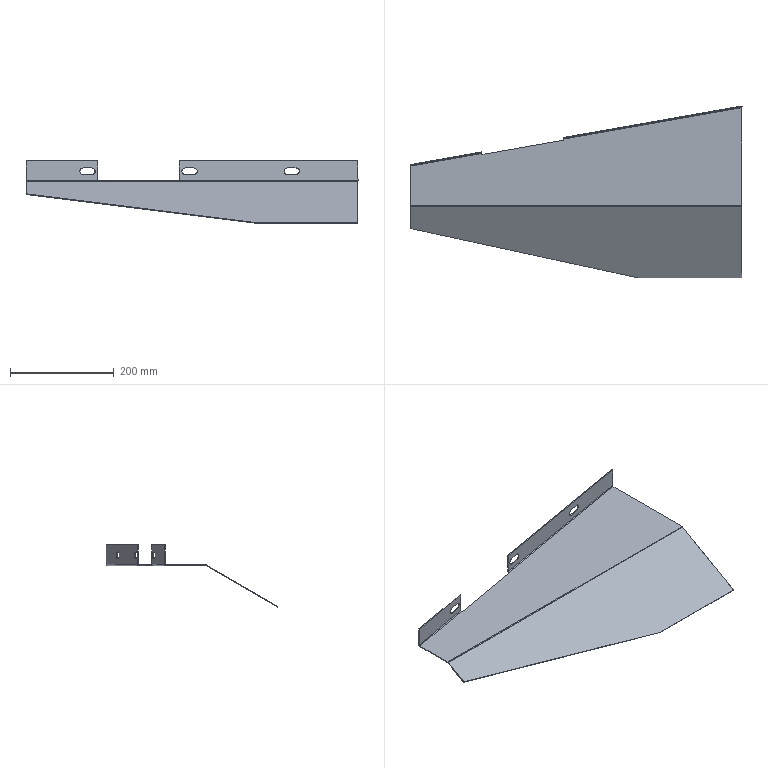Part | SolidWorks | features BaseBody 1 | 1 solid | 42 faces | box 640.37 x 331.413 x 119.799 mm | volume 272644 mm3 | plane 25 | cylinder 15 | spline 2 | commonest cylinder face diameters 13 x9 3 x3 6 x3
STEP:
#1=CARTESIAN_POINT('',(-193.452,62.314,26.5));
#2=VERTEX_POINT('',#1);
#3=CARTESIAN_POINT('',(-187.051,63.443,20.));
#4=VERTEX_POINT('',#3);
#5=CARTESIAN_POINT('',(-193.452,62.314,20.));
#6=DIRECTION('',(-0.1736,0.9848,0.));
#7=DIRECTION('',(0.9848,0.1736,0.));
#8=AXIS2_PLACEMENT_3D('',#5,#6,#7);
#9=CIRCLE('',#8,6.5);
#10=EDGE_CURVE('',#2,#4,#9,.T.);
#11=ORIENTED_EDGE('',*,*,#10,.T.);
#12=CARTESIAN_POINT('',(-186.79,61.965,20.));
#13=VERTEX_POINT('',#12);
#14=CARTESIAN_POINT('',(-187.051,63.443,20.));
#15=DIRECTION('',(0.1736,-0.9848,0.));
#16=VECTOR('',#15,1000.);
#17=LINE('',#14,#16);
#18=EDGE_CURVE('',#4,#13,#17,.T.);
#19=ORIENTED_EDGE('',*,*,#18,.T.);
#20=CARTESIAN_POINT('',(-193.192,60.837,26.5));
#21=VERTEX_POINT('',#20);
#22=CARTESIAN_POINT('',(-193.192,60.837,20.));
#23=DIRECTION('',(-0.1736,0.9848,0.));
#24=DIRECTION('',(0.9848,0.1736,0.));
#25=AXIS2_PLACEMENT_3D('',#22,#23,#24);
#26=CIRCLE('',#25,6.5);
#27=EDGE_CURVE('',#21,#13,#26,.T.);
#28=ORIENTED_EDGE('',*,*,#27,.F.);
#29=CARTESIAN_POINT('',(-193.452,62.314,26.5));
#30=DIRECTION('',(0.1736,-0.9848,0.));
#31=VECTOR('',#30,1000.);
#32=LINE('',#29,#31);
#33=EDGE_CURVE('',#2,#21,#32,.T.);
#34=ORIENTED_EDGE('',*,*,#33,.F.);
#35=EDGE_LOOP('',(#11,#19,#28,#34));
#36=FACE_OUTER_BOUND('',#35,.T.);
#37=CARTESIAN_POINT('',(-193.452,62.314,20.));
#38=DIRECTION('',(0.1736,-0.9848,0.));
#39=DIRECTION('',(0.9848,0.1736,0.));
#40=AXIS2_PLACEMENT_3D('',#37,#38,#39);
#41=CYLINDRICAL_SURFACE('',#40,6.5);
#42=ADVANCED_FACE('',(#36),#41,.F.);
#43=CARTESIAN_POINT('',(3.509,97.043,26.5));
#44=VERTEX_POINT('',#43);
#45=CARTESIAN_POINT('',(9.911,98.172,20.));
#46=VERTEX_POINT('',#45);
#47=CARTESIAN_POINT('',(3.509,97.043,20.));
#48=DIRECTION('',(-0.1736,0.9848,0.));
#49=DIRECTION('',(0.9848,0.1736,0.));
#50=AXIS2_PLACEMENT_3D('',#47,#48,#49);
#51=CIRCLE('',#50,6.5);
#52=EDGE_CURVE('',#44,#46,#51,.T.);
#53=ORIENTED_EDGE('',*,*,#52,.T.);
#54=CARTESIAN_POINT('',(10.171,96.695,20.));
#55=VERTEX_POINT('',#54);
#56=CARTESIAN_POINT('',(9.911,98.172,20.));
#57=DIRECTION('',(0.1736,-0.9848,0.));
#58=VECTOR('',#57,1000.);
#59=LINE('',#56,#58);
#60=EDGE_CURVE('',#46,#55,#59,.T.);
#61=ORIENTED_EDGE('',*,*,#60,.T.);
#62=CARTESIAN_POINT('',(3.77,95.566,26.5));
#63=VERTEX_POINT('',#62);
#64=CARTESIAN_POINT('',(3.77,95.566,20.));
#65=DIRECTION('',(-0.1736,0.9848,0.));
#66=DIRECTION('',(0.9848,0.1736,0.));
#67=AXIS2_PLACEMENT_3D('',#64,#65,#66);
#68=CIRCLE('',#67,6.5);
#69=EDGE_CURVE('',#63,#55,#68,.T.);
#70=ORIENTED_EDGE('',*,*,#69,.F.);
#71=CARTESIAN_POINT('',(3.77,95.566,26.5));
#72=DIRECTION('',(-0.1736,0.9848,0.));
#73=VECTOR('',#72,1000.);
#74=LINE('',#71,#73);
#75=EDGE_CURVE('',#63,#44,#74,.T.);
#76=ORIENTED_EDGE('',*,*,#75,.T.);
#77=EDGE_LOOP('',(#53,#61,#70,#76));
#78=FACE_OUTER_BOUND('',#77,.T.);
#79=CARTESIAN_POINT('',(3.509,97.043,20.));
#80=DIRECTION('',(0.1736,-0.9848,0.));
#81=DIRECTION('',(0.9848,0.1736,0.));
#82=AXIS2_PLACEMENT_3D('',#79,#80,#81);
#83=CYLINDRICAL_SURFACE('',#82,6.5);
#84=ADVANCED_FACE('',(#78),#83,.F.);
#85=CARTESIAN_POINT('',(200.471,131.773,26.5));
#86=VERTEX_POINT('',#85);
#87=CARTESIAN_POINT('',(206.872,132.902,20.));
#88=VERTEX_POINT('',#87);
#89=CARTESIAN_POINT('',(200.471,131.773,20.));
#90=DIRECTION('',(-0.1736,0.9848,0.));
#91=DIRECTION('',(0.9848,0.1736,0.));
#92=AXIS2_PLACEMENT_3D('',#89,#90,#91);
#93=CIRCLE('',#92,6.5);
#94=EDGE_CURVE('',#86,#88,#93,.T.);
#95=ORIENTED_EDGE('',*,*,#94,.T.);
#96=CARTESIAN_POINT('',(207.133,131.425,20.));
#97=VERTEX_POINT('',#96);
#98=CARTESIAN_POINT('',(206.872,132.902,20.));
#99=DIRECTION('',(0.1736,-0.9848,0.));
#100=VECTOR('',#99,1000.);
#101=LINE('',#98,#100);
#102=EDGE_CURVE('',#88,#97,#101,.T.);
#103=ORIENTED_EDGE('',*,*,#102,.T.);
#104=CARTESIAN_POINT('',(200.731,130.296,26.5));
#105=VERTEX_POINT('',#104);
#106=CARTESIAN_POINT('',(200.731,130.296,20.));
#107=DIRECTION('',(-0.1736,0.9848,0.));
#108=DIRECTION('',(0.9848,0.1736,0.));
#109=AXIS2_PLACEMENT_3D('',#106,#107,#108);
#110=CIRCLE('',#109,6.5);
#111=EDGE_CURVE('',#105,#97,#110,.T.);
#112=ORIENTED_EDGE('',*,*,#111,.F.);
#113=CARTESIAN_POINT('',(200.731,130.296,26.5));
#114=DIRECTION('',(-0.1736,0.9848,0.));
#115=VECTOR('',#114,1000.);
#116=LINE('',#113,#115);
#117=EDGE_CURVE('',#105,#86,#116,.T.);
#118=ORIENTED_EDGE('',*,*,#117,.T.);
#119=EDGE_LOOP('',(#95,#103,#112,#118));
#120=FACE_OUTER_BOUND('',#119,.T.);
#121=CARTESIAN_POINT('',(200.471,131.773,20.));
#122=DIRECTION('',(0.1736,-0.9848,0.));
#123=DIRECTION('',(0.9848,0.1736,0.));
#124=AXIS2_PLACEMENT_3D('',#121,#122,#123);
#125=CYLINDRICAL_SURFACE('',#124,6.5);
#126=ADVANCED_FACE('',(#120),#125,.F.);
#127=CARTESIAN_POINT('',(-23.689,87.17,0.));
#128=VERTEX_POINT('',#127);
#129=CARTESIAN_POINT('',(-181.259,59.387,0.));
#130=VERTEX_POINT('',#129);
#131=CARTESIAN_POINT('',(-23.689,87.17,0.));
#132=DIRECTION('',(-0.9848,-0.1736,0.));
#133=VECTOR('',#132,1000.);
#134=LINE('',#131,#133);
#135=EDGE_CURVE('',#128,#130,#134,.T.);
#136=ORIENTED_EDGE('',*,*,#135,.F.);
#137=CARTESIAN_POINT('',(-24.037,89.14,0.));
#138=VERTEX_POINT('',#137);
#139=CARTESIAN_POINT('',(-24.037,89.14,0.));
#140=DIRECTION('',(0.1736,-0.9848,0.));
#141=VECTOR('',#140,1000.);
#142=LINE('',#139,#141);
#143=EDGE_CURVE('',#138,#128,#142,.T.);
#144=ORIENTED_EDGE('',*,*,#143,.F.);
#145=CARTESIAN_POINT('',(320.,149.803,0.));
#146=VERTEX_POINT('',#145);
#147=CARTESIAN_POINT('',(320.,149.803,0.));
#148=DIRECTION('',(-0.9848,-0.1736,0.));
#149=VECTOR('',#148,1000.);
#150=LINE('',#147,#149);
#151=EDGE_CURVE('',#146,#138,#150,.T.);
#152=ORIENTED_EDGE('',*,*,#151,.F.);
#153=CARTESIAN_POINT('',(320.,-39.196,0.));
#154=VERTEX_POINT('',#153);
#155=CARTESIAN_POINT('',(320.,30.681,0.));
#156=DIRECTION('',(0.,1.,0.));
#157=VECTOR('',#156,1000.);
#158=LINE('',#155,#157);
#159=EDGE_CURVE('',#154,#146,#158,.T.);
#160=ORIENTED_EDGE('',*,*,#159,.F.);
#161=CARTESIAN_POINT('',(-320.,-39.196,0.));
#162=VERTEX_POINT('',#161);
#163=CARTESIAN_POINT('',(23.108,-39.196,0.));
#164=DIRECTION('',(1.,0.,0.));
#165=VECTOR('',#164,1000.);
#166=LINE('',#163,#165);
#167=EDGE_CURVE('',#162,#154,#166,.T.);
#168=ORIENTED_EDGE('',*,*,#167,.F.);
#169=CARTESIAN_POINT('',(-320.,36.954,0.));
#170=VERTEX_POINT('',#169);
#171=CARTESIAN_POINT('',(-320.,30.681,0.));
#172=DIRECTION('',(0.,-1.,0.));
#173=VECTOR('',#172,1000.);
#174=LINE('',#171,#173);
#175=EDGE_CURVE('',#170,#162,#174,.T.);
#176=ORIENTED_EDGE('',*,*,#175,.F.);
#177=CARTESIAN_POINT('',(-181.606,61.356,0.));
#178=VERTEX_POINT('',#177);
#179=CARTESIAN_POINT('',(-181.606,61.356,0.));
#180=DIRECTION('',(-0.9848,-0.1736,0.));
#181=VECTOR('',#180,1000.);
#182=LINE('',#179,#181);
#183=EDGE_CURVE('',#178,#170,#182,.T.);
#184=ORIENTED_EDGE('',*,*,#183,.F.);
#185=CARTESIAN_POINT('',(-181.259,59.387,0.));
#186=DIRECTION('',(-0.1736,0.9848,0.));
#187=VECTOR('',#186,1000.);
#188=LINE('',#185,#187);
#189=EDGE_CURVE('',#130,#178,#188,.T.);
#190=ORIENTED_EDGE('',*,*,#189,.F.);
#191=EDGE_LOOP('',(#136,#144,#152,#160,#168,#176,#184,#190));
#192=FACE_OUTER_BOUND('',#191,.T.);
#193=CARTESIAN_POINT('',(23.108,30.681,0.));
#194=DIRECTION('',(0.,0.,1.));
#195=DIRECTION('',(1.,0.,0.));
#196=AXIS2_PLACEMENT_3D('',#193,#194,#195);
#197=PLANE('',#196);
#198=ADVANCED_FACE('',(#192),#197,.F.);
#199=CARTESIAN_POINT('',(-182.127,64.311,3.));
#200=VERTEX_POINT('',#199);
#201=CARTESIAN_POINT('',(-181.606,61.356,3.));
#202=DIRECTION('',(-0.9848,-0.1736,0.));
#203=DIRECTION('',(-0.1736,0.9848,0.));
#204=AXIS2_PLACEMENT_3D('',#201,#202,#203);
#205=CIRCLE('',#204,3.);
#206=EDGE_CURVE('',#200,#178,#205,.T.);
#207=ORIENTED_EDGE('',*,*,#206,.F.);
#208=CARTESIAN_POINT('',(-182.127,64.311,40.));
#209=VERTEX_POINT('',#208);
#210=CARTESIAN_POINT('',(-182.127,64.311,55.));
#211=DIRECTION('',(0.,0.,-1.));
#212=VECTOR('',#211,1000.);
#213=LINE('',#210,#212);
#214=EDGE_CURVE('',#209,#200,#213,.T.);
#215=ORIENTED_EDGE('',*,*,#214,.F.);
#216=CARTESIAN_POINT('',(-181.866,62.834,40.));
#217=VERTEX_POINT('',#216);
#218=CARTESIAN_POINT('',(-181.866,62.834,40.));
#219=DIRECTION('',(-0.1736,0.9848,0.));
#220=VECTOR('',#219,1000.);
#221=LINE('',#218,#220);
#222=EDGE_CURVE('',#217,#209,#221,.T.);
#223=ORIENTED_EDGE('',*,*,#222,.F.);
#224=CARTESIAN_POINT('',(-181.866,62.834,3.));
#225=VERTEX_POINT('',#224);
#226=CARTESIAN_POINT('',(-181.866,62.834,55.));
#227=DIRECTION('',(0.,0.,1.));
#228=VECTOR('',#227,1000.);
#229=LINE('',#226,#228);
#230=EDGE_CURVE('',#225,#217,#229,.T.);
#231=ORIENTED_EDGE('',*,*,#230,.F.);
#232=CARTESIAN_POINT('',(-181.606,61.356,1.5));
#233=VERTEX_POINT('',#232);
#234=CARTESIAN_POINT('',(-181.606,61.356,3.));
#235=DIRECTION('',(0.9848,0.1736,0.));
#236=DIRECTION('',(-0.1736,0.9848,0.));
#237=AXIS2_PLACEMENT_3D('',#234,#235,#236);
#238=CIRCLE('',#237,1.5);
#239=EDGE_CURVE('',#233,#225,#238,.T.);
#240=ORIENTED_EDGE('',*,*,#239,.F.);
#241=CARTESIAN_POINT('',(-181.259,59.387,1.5));
#242=VERTEX_POINT('',#241);
#243=CARTESIAN_POINT('',(-182.127,64.311,1.5));
#244=DIRECTION('',(-0.1736,0.9848,0.));
#245=VECTOR('',#244,1000.);
#246=LINE('',#243,#245);
#247=EDGE_CURVE('',#242,#233,#246,.T.);
#248=ORIENTED_EDGE('',*,*,#247,.F.);
#249=CARTESIAN_POINT('',(-181.259,59.387,55.));
#250=DIRECTION('',(0.,0.,1.));
#251=VECTOR('',#250,1000.);
#252=LINE('',#249,#251);
#253=EDGE_CURVE('',#130,#242,#252,.T.);
#254=ORIENTED_EDGE('',*,*,#253,.F.);
#255=ORIENTED_EDGE('',*,*,#189,.T.);
#256=EDGE_LOOP('',(#207,#215,#223,#231,#240,#248,#254,#255));
#257=FACE_OUTER_BOUND('',#256,.T.);
#258=CARTESIAN_POINT('',(-182.127,64.311,55.));
#259=DIRECTION('',(-0.9848,-0.1736,0.));
#260=DIRECTION('',(0.1736,-0.9848,0.));
#261=AXIS2_PLACEMENT_3D('',#258,#259,#260);
#262=PLANE('',#261);
#263=ADVANCED_FACE('',(#257),#262,.F.);
#264=ORIENTED_EDGE('',*,*,#253,.T.);
#265=CARTESIAN_POINT('',(-23.689,87.17,1.5));
#266=VERTEX_POINT('',#265);
#267=CARTESIAN_POINT('',(-102.474,73.279,1.5));
#268=DIRECTION('',(-0.9848,-0.1736,0.));
#269=VECTOR('',#268,1000.);
#270=LINE('',#267,#269);
#271=EDGE_CURVE('',#266,#242,#270,.T.);
#272=ORIENTED_EDGE('',*,*,#271,.F.);
#273=CARTESIAN_POINT('',(-23.689,87.17,25.));
#274=DIRECTION('',(0.,0.,1.));
#275=VECTOR('',#274,1000.);
#276=LINE('',#273,#275);
#277=EDGE_CURVE('',#128,#266,#276,.T.);
#278=ORIENTED_EDGE('',*,*,#277,.F.);
#279=ORIENTED_EDGE('',*,*,#135,.T.);
#280=EDGE_LOOP('',(#264,#272,#278,#279));
#281=FACE_OUTER_BOUND('',#280,.T.);
#282=CARTESIAN_POINT('',(-102.474,73.279,25.));
#283=DIRECTION('',(0.1736,-0.9848,0.));
#284=DIRECTION('',(0.9848,0.1736,0.));
#285=AXIS2_PLACEMENT_3D('',#282,#283,#284);
#286=PLANE('',#285);
#287=ADVANCED_FACE('',(#281),#286,.F.);
#288=ORIENTED_EDGE('',*,*,#277,.T.);
#289=CARTESIAN_POINT('',(-24.037,89.14,1.5));
#290=VERTEX_POINT('',#289);
#291=CARTESIAN_POINT('',(-24.558,92.094,1.5));
#292=DIRECTION('',(0.1736,-0.9848,0.));
#293=VECTOR('',#292,1000.);
#294=LINE('',#291,#293);
#295=EDGE_CURVE('',#290,#266,#294,.T.);
#296=ORIENTED_EDGE('',*,*,#295,.F.);
#297=CARTESIAN_POINT('',(-24.297,90.617,3.));
#298=VERTEX_POINT('',#297);
#299=CARTESIAN_POINT('',(-24.037,89.14,3.));
#300=DIRECTION('',(-0.9848,-0.1736,0.));
#301=DIRECTION('',(-0.1736,0.9848,0.));
#302=AXIS2_PLACEMENT_3D('',#299,#300,#301);
#303=CIRCLE('',#302,1.5);
#304=EDGE_CURVE('',#298,#290,#303,.T.);
#305=ORIENTED_EDGE('',*,*,#304,.F.);
#306=CARTESIAN_POINT('',(-24.297,90.617,40.));
#307=VERTEX_POINT('',#306);
#308=CARTESIAN_POINT('',(-24.297,90.617,-5.));
#309=DIRECTION('',(0.,0.,-1.));
#310=VECTOR('',#309,1000.);
#311=LINE('',#308,#310);
#312=EDGE_CURVE('',#307,#298,#311,.T.);
#313=ORIENTED_EDGE('',*,*,#312,.F.);
#314=CARTESIAN_POINT('',(-24.558,92.094,40.));
#315=VERTEX_POINT('',#314);
#316=CARTESIAN_POINT('',(-24.558,92.094,40.));
#317=DIRECTION('',(0.1736,-0.9848,0.));
#318=VECTOR('',#317,1000.);
#319=LINE('',#316,#318);
#320=EDGE_CURVE('',#315,#307,#319,.T.);
#321=ORIENTED_EDGE('',*,*,#320,.F.);
#322=CARTESIAN_POINT('',(-24.558,92.094,3.));
#323=VERTEX_POINT('',#322);
#324=CARTESIAN_POINT('',(-24.558,92.094,-5.));
#325=DIRECTION('',(0.,0.,1.));
#326=VECTOR('',#325,1000.);
#327=LINE('',#324,#326);
#328=EDGE_CURVE('',#323,#315,#327,.T.);
#329=ORIENTED_EDGE('',*,*,#328,.F.);
#330=CARTESIAN_POINT('',(-24.037,89.14,3.));
#331=DIRECTION('',(0.9848,0.1736,0.));
#332=DIRECTION('',(-0.1736,0.9848,0.));
#333=AXIS2_PLACEMENT_3D('',#330,#331,#332);
#334=CIRCLE('',#333,3.);
#335=EDGE_CURVE('',#138,#323,#334,.T.);
#336=ORIENTED_EDGE('',*,*,#335,.F.);
#337=ORIENTED_EDGE('',*,*,#143,.T.);
#338=EDGE_LOOP('',(#288,#296,#305,#313,#321,#329,#336,#337));
#339=FACE_OUTER_BOUND('',#338,.T.);
#340=CARTESIAN_POINT('',(-24.558,92.094,-5.));
#341=DIRECTION('',(0.9848,0.1736,0.));
#342=DIRECTION('',(-0.1736,0.9848,0.));
#343=AXIS2_PLACEMENT_3D('',#340,#341,#342);
#344=PLANE('',#343);
#345=ADVANCED_FACE('',(#339),#344,.F.);
#346=CARTESIAN_POINT('',(320.,152.849,3.));
#347=VERTEX_POINT('',#346);
#348=CARTESIAN_POINT('',(320.,152.849,3.));
#349=CARTESIAN_POINT('',(319.978,152.845,2.802));
#350=CARTESIAN_POINT('',(319.96,152.822,2.607));
#351=CARTESIAN_POINT('',(319.93,152.739,2.221));
#352=CARTESIAN_POINT('',(319.918,152.678,2.031));
#353=CARTESIAN_POINT('',(319.901,152.523,1.67));
#354=CARTESIAN_POINT('',(319.895,152.429,1.497));
#355=CARTESIAN_POINT('',(319.89,152.205,1.169));
#356=CARTESIAN_POINT('',(319.89,152.078,1.017));
#357=CARTESIAN_POINT('',(319.894,151.798,0.7407));
#358=CARTESIAN_POINT('',(319.899,151.644,0.6153));
#359=CARTESIAN_POINT('',(319.912,151.314,0.3961));
#360=CARTESIAN_POINT('',(319.921,151.14,0.3041));
#361=CARTESIAN_POINT('',(319.94,150.777,0.1542));
#362=CARTESIAN_POINT('',(319.952,150.585,0.09621));
#363=CARTESIAN_POINT('',(319.975,150.198,0.01942));
#364=CARTESIAN_POINT('',(319.988,150.002,0.));
#365=CARTESIAN_POINT('',(320.,149.803,0.));
#366=B_SPLINE_CURVE_WITH_KNOTS('',3,(#348,#349,#350,#351,#352,#353,#354,#355,#356,#357,#358,#359,#360,#361,#362,#363,#364,#365),.UNSPECIFIED.,.F.,.F.,(4,2,2,2,2,2,2,2,4),(0.,0.000592,0.001184,0.001776,0.002368,0.00296,0.003552,0.004144,0.004736),.UNSPECIFIED.);
#367=EDGE_CURVE('',#347,#146,#366,.T.);
#368=ORIENTED_EDGE('',*,*,#367,.T.);
#369=ORIENTED_EDGE('',*,*,#151,.T.);
#370=ORIENTED_EDGE('',*,*,#335,.T.);
#371=CARTESIAN_POINT('',(-0.5209,96.333,3.));
#372=DIRECTION('',(0.9848,0.1736,0.));
#373=VECTOR('',#372,1000.);
#374=LINE('',#371,#373);
#375=EDGE_CURVE('',#323,#347,#374,.T.);
#376=ORIENTED_EDGE('',*,*,#375,.T.);
#377=EDGE_LOOP('',(#368,#369,#370,#376));
#378=FACE_OUTER_BOUND('',#377,.T.);
#379=CARTESIAN_POINT('',(0.,93.378,3.));
#380=DIRECTION('',(0.9848,0.1736,0.));
#381=DIRECTION('',(-0.1736,0.9848,0.));
#382=AXIS2_PLACEMENT_3D('',#379,#380,#381);
#383=CYLINDRICAL_SURFACE('',#382,3.);
#384=ADVANCED_FACE('',(#378),#383,.T.);
#385=CARTESIAN_POINT('',(320.,149.803,1.5));
#386=VERTEX_POINT('',#385);
#387=CARTESIAN_POINT('',(320.,149.803,0.));
#388=DIRECTION('',(0.,0.,1.));
#389=VECTOR('',#388,1000.);
#390=LINE('',#387,#389);
#391=EDGE_CURVE('',#146,#386,#390,.T.);
#392=ORIENTED_EDGE('',*,*,#391,.T.);
#393=CARTESIAN_POINT('',(320.,-39.196,1.5));
#394=VERTEX_POINT('',#393);
#395=CARTESIAN_POINT('',(320.,40.,1.5));
#396=DIRECTION('',(0.,-1.,0.));
#397=VECTOR('',#396,1000.);
#398=LINE('',#395,#397);
#399=EDGE_CURVE('',#386,#394,#398,.T.);
#400=ORIENTED_EDGE('',*,*,#399,.T.);
#401=CARTESIAN_POINT('',(320.,-40.696,1.098));
#402=VERTEX_POINT('',#401);
#403=CARTESIAN_POINT('',(320.,-39.196,-1.5));
#404=DIRECTION('',(1.,0.,0.));
#405=DIRECTION('',(0.,1.,0.));
#406=AXIS2_PLACEMENT_3D('',#403,#404,#405);
#407=CIRCLE('',#406,3.);
#408=EDGE_CURVE('',#394,#402,#407,.T.);
#409=ORIENTED_EDGE('',*,*,#408,.T.);
#410=CARTESIAN_POINT('',(320.,-178.564,-78.5));
#411=VERTEX_POINT('',#410);
#412=CARTESIAN_POINT('',(320.,-40.696,1.098));
#413=DIRECTION('',(0.,-0.866,-0.5));
#414=VECTOR('',#413,1000.);
#415=LINE('',#412,#414);
#416=EDGE_CURVE('',#402,#411,#415,.T.);
#417=ORIENTED_EDGE('',*,*,#416,.T.);
#418=CARTESIAN_POINT('',(320.,-177.814,-79.799));
#419=VERTEX_POINT('',#418);
#420=CARTESIAN_POINT('',(320.,-178.564,-78.5));
#421=DIRECTION('',(0.,0.5,-0.866));
#422=VECTOR('',#421,1000.);
#423=LINE('',#420,#422);
#424=EDGE_CURVE('',#411,#419,#423,.T.);
#425=ORIENTED_EDGE('',*,*,#424,.T.);
#426=CARTESIAN_POINT('',(320.,-39.946,-0.201));
#427=VERTEX_POINT('',#426);
#428=CARTESIAN_POINT('',(320.,-108.39,-39.717));
#429=DIRECTION('',(0.,0.866,0.5));
#430=VECTOR('',#429,1000.);
#431=LINE('',#428,#430);
#432=EDGE_CURVE('',#419,#427,#431,.T.);
#433=ORIENTED_EDGE('',*,*,#432,.T.);
#434=CARTESIAN_POINT('',(320.,-39.196,-1.5));
#435=DIRECTION('',(-1.,0.,0.));
#436=DIRECTION('',(0.,1.,0.));
#437=AXIS2_PLACEMENT_3D('',#434,#435,#436);
#438=CIRCLE('',#437,1.5);
#439=EDGE_CURVE('',#427,#154,#438,.T.);
#440=ORIENTED_EDGE('',*,*,#439,.T.);
#441=ORIENTED_EDGE('',*,*,#159,.T.);
#442=EDGE_LOOP('',(#392,#400,#409,#417,#425,#433,#440,#441));
#443=FACE_OUTER_BOUND('',#442,.T.);
#444=CARTESIAN_POINT('',(320.,40.,0.));
#445=DIRECTION('',(1.,0.,0.));
#446=DIRECTION('',(0.,0.,-1.));
#447=AXIS2_PLACEMENT_3D('',#444,#445,#446);
#448=PLANE('',#447);
#449=ADVANCED_FACE('',(#443),#448,.T.);
#450=CARTESIAN_POINT('',(-320.,-39.946,-0.201));
#451=VERTEX_POINT('',#450);
#452=CARTESIAN_POINT('',(-320.,-39.196,-1.5));
#453=DIRECTION('',(1.,0.,0.));
#454=DIRECTION('',(0.,1.,0.));
#455=AXIS2_PLACEMENT_3D('',#452,#453,#454);
#456=CIRCLE('',#455,1.5);
#457=EDGE_CURVE('',#162,#451,#456,.T.);
#458=ORIENTED_EDGE('',*,*,#457,.F.);
#459=ORIENTED_EDGE('',*,*,#167,.T.);
#460=ORIENTED_EDGE('',*,*,#439,.F.);
#461=CARTESIAN_POINT('',(0.,-39.946,-0.201));
#462=DIRECTION('',(1.,0.,0.));
#463=VECTOR('',#462,1000.);
#464=LINE('',#461,#463);
#465=EDGE_CURVE('',#451,#427,#464,.T.);
#466=ORIENTED_EDGE('',*,*,#465,.F.);
#467=EDGE_LOOP('',(#458,#459,#460,#466));
#468=FACE_OUTER_BOUND('',#467,.T.);
#469=CARTESIAN_POINT('',(0.,-39.196,-1.5));
#470=DIRECTION('',(1.,0.,0.));
#471=DIRECTION('',(0.,1.,0.));
#472=AXIS2_PLACEMENT_3D('',#469,#470,#471);
#473=CYLINDRICAL_SURFACE('',#472,1.5);
#474=ADVANCED_FACE('',(#468),#473,.F.);
#475=CARTESIAN_POINT('',(-320.,36.954,1.5));
#476=VERTEX_POINT('',#475);
#477=CARTESIAN_POINT('',(-320.,36.954,0.75));
#478=DIRECTION('',(0.,0.,1.));
#479=VECTOR('',#478,1000.);
#480=LINE('',#477,#479);
#481=EDGE_CURVE('',#170,#476,#480,.T.);
#482=ORIENTED_EDGE('',*,*,#481,.F.);
#483=ORIENTED_EDGE('',*,*,#175,.T.);
#484=ORIENTED_EDGE('',*,*,#457,.T.);
#485=CARTESIAN_POINT('',(-320.,-82.551,-24.799));
#486=VERTEX_POINT('',#485);
#487=CARTESIAN_POINT('',(-320.,-108.39,-39.717));
#488=DIRECTION('',(0.,-0.866,-0.5));
#489=VECTOR('',#488,1000.);
#490=LINE('',#487,#489);
#491=EDGE_CURVE('',#451,#486,#490,.T.);
#492=ORIENTED_EDGE('',*,*,#491,.T.);
#493=CARTESIAN_POINT('',(-320.,-83.301,-23.5));
#494=VERTEX_POINT('',#493);
#495=CARTESIAN_POINT('',(-320.,-83.301,-23.5));
#496=DIRECTION('',(0.,-0.5,0.866));
#497=VECTOR('',#496,1000.);
#498=LINE('',#495,#497);
#499=EDGE_CURVE('',#486,#494,#498,.T.);
#500=ORIENTED_EDGE('',*,*,#499,.T.);
#501=CARTESIAN_POINT('',(-320.,-40.696,1.098));
#502=VERTEX_POINT('',#501);
#503=CARTESIAN_POINT('',(-320.,-83.301,-23.5));
#504=DIRECTION('',(0.,0.866,0.5));
#505=VECTOR('',#504,1000.);
#506=LINE('',#503,#505);
#507=EDGE_CURVE('',#494,#502,#506,.T.);
#508=ORIENTED_EDGE('',*,*,#507,.T.);
#509=CARTESIAN_POINT('',(-320.,-39.196,1.5));
#510=VERTEX_POINT('',#509);
#511=CARTESIAN_POINT('',(-320.,-39.196,-1.5));
#512=DIRECTION('',(-1.,0.,0.));
#513=DIRECTION('',(0.,1.,0.));
#514=AXIS2_PLACEMENT_3D('',#511,#512,#513);
#515=CIRCLE('',#514,3.);
#516=EDGE_CURVE('',#502,#510,#515,.T.);
#517=ORIENTED_EDGE('',*,*,#516,.T.);
#518=CARTESIAN_POINT('',(-320.,-40.,1.5));
#519=DIRECTION('',(0.,1.,0.));
#520=VECTOR('',#519,1000.);
#521=LINE('',#518,#520);
#522=EDGE_CURVE('',#510,#476,#521,.T.);
#523=ORIENTED_EDGE('',*,*,#522,.T.);
#524=EDGE_LOOP('',(#482,#483,#484,#492,#500,#508,#517,#523));
#525=FACE_OUTER_BOUND('',#524,.T.);
#526=CARTESIAN_POINT('',(-320.,-40.,0.));
#527=DIRECTION('',(-1.,0.,0.));
#528=DIRECTION('',(0.,-1.,0.));
#529=AXIS2_PLACEMENT_3D('',#526,#527,#528);
#530=PLANE('',#529);
#531=ADVANCED_FACE('',(#525),#530,.T.);
#532=CARTESIAN_POINT('',(-320.,40.,3.));
#533=VERTEX_POINT('',#532);
#534=CARTESIAN_POINT('',(-320.,36.954,0.));
#535=CARTESIAN_POINT('',(-320.012,37.153,0.));
#536=CARTESIAN_POINT('',(-320.025,37.349,0.01942));
#537=CARTESIAN_POINT('',(-320.048,37.736,0.09615));
#538=CARTESIAN_POINT('',(-320.06,37.927,0.1542));
#539=CARTESIAN_POINT('',(-320.079,38.291,0.3041));
#540=CARTESIAN_POINT('',(-320.088,38.464,0.3961));
#541=CARTESIAN_POINT('',(-320.101,38.795,0.6151));
#542=CARTESIAN_POINT('',(-320.106,38.949,0.7406));
#543=CARTESIAN_POINT('',(-320.11,39.228,1.017));
#544=CARTESIAN_POINT('',(-320.11,39.356,1.169));
#545=CARTESIAN_POINT('',(-320.105,39.579,1.497));
#546=CARTESIAN_POINT('',(-320.099,39.674,1.67));
#547=CARTESIAN_POINT('',(-320.082,39.829,2.031));
#548=CARTESIAN_POINT('',(-320.07,39.89,2.221));
#549=CARTESIAN_POINT('',(-320.04,39.973,2.607));
#550=CARTESIAN_POINT('',(-320.022,39.996,2.802));
#551=CARTESIAN_POINT('',(-320.,40.,3.));
#552=B_SPLINE_CURVE_WITH_KNOTS('',3,(#534,#535,#536,#537,#538,#539,#540,#541,#542,#543,#544,#545,#546,#547,#548,#549,#550,#551),.UNSPECIFIED.,.F.,.F.,(4,2,2,2,2,2,2,2,4),(0.,0.000592,0.001184,0.001776,0.002368,0.00296,0.003552,0.004144,0.004736),.UNSPECIFIED.);
#553=EDGE_CURVE('',#170,#533,#552,.T.);
#554=ORIENTED_EDGE('',*,*,#553,.T.);
#555=CARTESIAN_POINT('',(-0.5209,96.333,3.));
#556=DIRECTION('',(0.9848,0.1736,0.));
#557=VECTOR('',#556,1000.);
#558=LINE('',#555,#557);
#559=EDGE_CURVE('',#533,#200,#558,.T.);
#560=ORIENTED_EDGE('',*,*,#559,.T.);
#561=ORIENTED_EDGE('',*,*,#206,.T.);
#562=ORIENTED_EDGE('',*,*,#183,.T.);
#563=EDGE_LOOP('',(#554,#560,#561,#562));
#564=FACE_OUTER_BOUND('',#563,.T.);
#565=CARTESIAN_POINT('',(0.,93.378,3.));
#566=DIRECTION('',(0.9848,0.1736,0.));
#567=DIRECTION('',(-0.1736,0.9848,0.));
#568=AXIS2_PLACEMENT_3D('',#565,#566,#567);
#569=CYLINDRICAL_SURFACE('',#568,3.);
#570=ADVANCED_FACE('',(#564),#569,.T.);
#571=CARTESIAN_POINT('',(-210.194,59.362,26.5));
#572=VERTEX_POINT('',#571);
#573=CARTESIAN_POINT('',(-0.2465,96.381,26.5));
#574=DIRECTION('',(0.9848,0.1736,0.));
#575=VECTOR('',#574,1000.);
#576=LINE('',#573,#575);
#577=EDGE_CURVE('',#572,#2,#576,.T.);
#578=ORIENTED_EDGE('',*,*,#577,.F.);
#579=CARTESIAN_POINT('',(-210.194,59.362,13.5));
#580=VERTEX_POINT('',#579);
#581=CARTESIAN_POINT('',(-210.194,59.362,20.));
#582=DIRECTION('',(-0.1736,0.9848,0.));
#583=DIRECTION('',(0.9848,0.1736,0.));
#584=AXIS2_PLACEMENT_3D('',#581,#582,#583);
#585=CIRCLE('',#584,6.5);
#586=EDGE_CURVE('',#580,#572,#585,.T.);
#587=ORIENTED_EDGE('',*,*,#586,.F.);
#588=CARTESIAN_POINT('',(-193.452,62.314,13.5));
#589=VERTEX_POINT('',#588);
#590=CARTESIAN_POINT('',(-0.2465,96.381,13.5));
#591=DIRECTION('',(-0.9848,-0.1736,0.));
#592=VECTOR('',#591,1000.);
#593=LINE('',#590,#592);
#594=EDGE_CURVE('',#589,#580,#593,.T.);
#595=ORIENTED_EDGE('',*,*,#594,.F.);
#596=CARTESIAN_POINT('',(-193.452,62.314,20.));
#597=DIRECTION('',(-0.1736,0.9848,0.));
#598=DIRECTION('',(0.9848,0.1736,0.));
#599=AXIS2_PLACEMENT_3D('',#596,#597,#598);
#600=CIRCLE('',#599,6.5);
#601=EDGE_CURVE('',#4,#589,#600,.T.);
#602=ORIENTED_EDGE('',*,*,#601,.F.);
#603=ORIENTED_EDGE('',*,*,#10,.F.);
#604=EDGE_LOOP('',(#578,#587,#595,#602,#603));
#605=FACE_BOUND('',#604,.T.);
#606=ORIENTED_EDGE('',*,*,#559,.F.);
#607=CARTESIAN_POINT('',(-320.,40.,40.));
#608=VERTEX_POINT('',#607);
#609=CARTESIAN_POINT('',(-320.,40.,19.802));
#610=DIRECTION('',(0.,0.,-1.));
#611=VECTOR('',#610,1000.);
#612=LINE('',#609,#611);
#613=EDGE_CURVE('',#608,#533,#612,.T.);
#614=ORIENTED_EDGE('',*,*,#613,.F.);
#615=CARTESIAN_POINT('',(-0.2465,96.381,40.));
#616=DIRECTION('',(-0.9848,-0.1736,0.));
#617=VECTOR('',#616,1000.);
#618=LINE('',#615,#617);
#619=EDGE_CURVE('',#209,#608,#618,.T.);
#620=ORIENTED_EDGE('',*,*,#619,.F.);
#621=ORIENTED_EDGE('',*,*,#214,.T.);
#622=EDGE_LOOP('',(#606,#614,#620,#621));
#623=FACE_OUTER_BOUND('',#622,.T.);
#624=CARTESIAN_POINT('',(-0.2465,96.381,19.802));
#625=DIRECTION('',(0.1736,-0.9848,0.));
#626=DIRECTION('',(0.9848,0.1736,0.));
#627=AXIS2_PLACEMENT_3D('',#624,#625,#626);
#628=PLANE('',#627);
#629=ADVANCED_FACE('',(#605,#623),#628,.F.);
#630=CARTESIAN_POINT('',(-209.933,57.885,13.5));
#631=VERTEX_POINT('',#630);
#632=CARTESIAN_POINT('',(-209.933,57.885,26.5));
#633=VERTEX_POINT('',#632);
#634=CARTESIAN_POINT('',(-209.933,57.885,20.));
#635=DIRECTION('',(-0.1736,0.9848,0.));
#636=DIRECTION('',(0.9848,0.1736,0.));
#637=AXIS2_PLACEMENT_3D('',#634,#635,#636);
#638=CIRCLE('',#637,6.5);
#639=EDGE_CURVE('',#631,#633,#638,.T.);
#640=ORIENTED_EDGE('',*,*,#639,.T.);
#641=CARTESIAN_POINT('',(0.01396,94.904,26.5));
#642=DIRECTION('',(0.9848,0.1736,0.));
#643=VECTOR('',#642,1000.);
#644=LINE('',#641,#643);
#645=EDGE_CURVE('',#633,#21,#644,.T.);
#646=ORIENTED_EDGE('',*,*,#645,.T.);
#647=ORIENTED_EDGE('',*,*,#27,.T.);
#648=CARTESIAN_POINT('',(-193.192,60.837,13.5));
#649=VERTEX_POINT('',#648);
#650=CARTESIAN_POINT('',(-193.192,60.837,20.));
#651=DIRECTION('',(-0.1736,0.9848,0.));
#652=DIRECTION('',(0.9848,0.1736,0.));
#653=AXIS2_PLACEMENT_3D('',#650,#651,#652);
#654=CIRCLE('',#653,6.5);
#655=EDGE_CURVE('',#13,#649,#654,.T.);
#656=ORIENTED_EDGE('',*,*,#655,.T.);
#657=CARTESIAN_POINT('',(0.01396,94.904,13.5));
#658=DIRECTION('',(-0.9848,-0.1736,0.));
#659=VECTOR('',#658,1000.);
#660=LINE('',#657,#659);
#661=EDGE_CURVE('',#649,#631,#660,.T.);
#662=ORIENTED_EDGE('',*,*,#661,.T.);
#663=EDGE_LOOP('',(#640,#646,#647,#656,#662));
#664=FACE_BOUND('',#663,.T.);
#665=CARTESIAN_POINT('',(-319.74,38.523,40.));
#666=VERTEX_POINT('',#665);
#667=CARTESIAN_POINT('',(-319.74,38.523,3.));
#668=VERTEX_POINT('',#667);
#669=CARTESIAN_POINT('',(-319.74,38.523,19.802));
#670=DIRECTION('',(0.,0.,-1.));
#671=VECTOR('',#670,1000.);
#672=LINE('',#669,#671);
#673=EDGE_CURVE('',#666,#668,#672,.T.);
#674=ORIENTED_EDGE('',*,*,#673,.T.);
#675=CARTESIAN_POINT('',(0.01396,94.904,3.));
#676=DIRECTION('',(0.9848,0.1736,0.));
#677=VECTOR('',#676,1000.);
#678=LINE('',#675,#677);
#679=EDGE_CURVE('',#668,#225,#678,.T.);
#680=ORIENTED_EDGE('',*,*,#679,.T.);
#681=ORIENTED_EDGE('',*,*,#230,.T.);
#682=CARTESIAN_POINT('',(0.01396,94.904,40.));
#683=DIRECTION('',(-0.9848,-0.1736,0.));
#684=VECTOR('',#683,1000.);
#685=LINE('',#682,#684);
#686=EDGE_CURVE('',#217,#666,#685,.T.);
#687=ORIENTED_EDGE('',*,*,#686,.T.);
#688=EDGE_LOOP('',(#674,#680,#681,#687));
#689=FACE_OUTER_BOUND('',#688,.T.);
#690=CARTESIAN_POINT('',(0.01396,94.904,19.802));
#691=DIRECTION('',(0.1736,-0.9848,0.));
#692=DIRECTION('',(0.9848,0.1736,0.));
#693=AXIS2_PLACEMENT_3D('',#690,#691,#692);
#694=PLANE('',#693);
#695=ADVANCED_FACE('',(#664,#689),#694,.T.);
#696=ORIENTED_EDGE('',*,*,#679,.F.);
#697=CARTESIAN_POINT('',(-320.,36.954,1.5));
#698=CARTESIAN_POINT('',(-319.991,37.157,1.5));
#699=CARTESIAN_POINT('',(-319.981,37.355,1.539));
#700=CARTESIAN_POINT('',(-319.964,37.635,1.652));
#701=CARTESIAN_POINT('',(-319.957,37.724,1.698));
#702=CARTESIAN_POINT('',(-319.942,37.892,1.806));
#703=CARTESIAN_POINT('',(-319.933,37.972,1.87));
#704=CARTESIAN_POINT('',(-319.914,38.116,2.008));
#705=CARTESIAN_POINT('',(-319.903,38.181,2.084));
#706=CARTESIAN_POINT('',(-319.879,38.296,2.247));
#707=CARTESIAN_POINT('',(-319.865,38.346,2.335));
#708=CARTESIAN_POINT('',(-319.82,38.468,2.605));
#709=CARTESIAN_POINT('',(-319.783,38.515,2.802));
#710=CARTESIAN_POINT('',(-319.74,38.523,3.));
#711=B_SPLINE_CURVE_WITH_KNOTS('',3,(#697,#698,#699,#700,#701,#702,#703,#704,#705,#706,#707,#708,#709,#710),.UNSPECIFIED.,.F.,.F.,(4,2,2,2,2,2,4),(0.,0.0006004,0.0009005,0.001201,0.001501,0.001801,0.002401),.UNSPECIFIED.);
#712=EDGE_CURVE('',#476,#668,#711,.T.);
#713=ORIENTED_EDGE('',*,*,#712,.F.);
#714=CARTESIAN_POINT('',(0.,93.378,1.5));
#715=DIRECTION('',(-0.9848,-0.1736,0.));
#716=VECTOR('',#715,1000.);
#717=LINE('',#714,#716);
#718=EDGE_CURVE('',#233,#476,#717,.T.);
#719=ORIENTED_EDGE('',*,*,#718,.F.);
#720=ORIENTED_EDGE('',*,*,#239,.T.);
#721=EDGE_LOOP('',(#696,#713,#719,#720));
#722=FACE_OUTER_BOUND('',#721,.T.);
#723=CARTESIAN_POINT('',(0.,93.378,3.));
#724=DIRECTION('',(0.9848,0.1736,0.));
#725=DIRECTION('',(-0.1736,0.9848,0.));
#726=AXIS2_PLACEMENT_3D('',#723,#724,#725);
#727=CYLINDRICAL_SURFACE('',#726,1.5);
#728=ADVANCED_FACE('',(#722),#727,.F.);
#729=ORIENTED_EDGE('',*,*,#295,.T.);
#730=ORIENTED_EDGE('',*,*,#271,.T.);
#731=ORIENTED_EDGE('',*,*,#247,.T.);
#732=ORIENTED_EDGE('',*,*,#718,.T.);
#733=ORIENTED_EDGE('',*,*,#522,.F.);
#734=CARTESIAN_POINT('',(23.108,-39.196,1.5));
#735=DIRECTION('',(1.,0.,0.));
#736=VECTOR('',#735,1000.);
#737=LINE('',#734,#736);
#738=EDGE_CURVE('',#510,#394,#737,.T.);
#739=ORIENTED_EDGE('',*,*,#738,.T.);
#740=ORIENTED_EDGE('',*,*,#399,.F.);
#741=CARTESIAN_POINT('',(320.,149.803,1.5));
#742=DIRECTION('',(-0.9848,-0.1736,0.));
#743=VECTOR('',#742,1000.);
#744=LINE('',#741,#743);
#745=EDGE_CURVE('',#386,#290,#744,.T.);
#746=ORIENTED_EDGE('',*,*,#745,.T.);
#747=EDGE_LOOP('',(#729,#730,#731,#732,#733,#739,#740,#746));
#748=FACE_OUTER_BOUND('',#747,.T.);
#749=CARTESIAN_POINT('',(23.108,30.681,1.5));
#750=DIRECTION('',(0.,0.,1.));
#751=DIRECTION('',(1.,0.,0.));
#752=AXIS2_PLACEMENT_3D('',#749,#750,#751);
#753=PLANE('',#752);
#754=ADVANCED_FACE('',(#748),#753,.T.);
#755=ORIENTED_EDGE('',*,*,#745,.F.);
#756=CARTESIAN_POINT('',(320.26,151.372,3.));
#757=VERTEX_POINT('',#756);
#758=CARTESIAN_POINT('',(320.26,151.372,3.));
#759=CARTESIAN_POINT('',(320.217,151.364,2.802));
#760=CARTESIAN_POINT('',(320.18,151.318,2.608));
#761=CARTESIAN_POINT('',(320.135,151.196,2.335));
#762=CARTESIAN_POINT('',(320.121,151.147,2.249));
#763=CARTESIAN_POINT('',(320.097,151.032,2.086));
#764=CARTESIAN_POINT('',(320.086,150.966,2.009));
#765=CARTESIAN_POINT('',(320.067,150.822,1.87));
#766=CARTESIAN_POINT('',(320.058,150.744,1.808));
#767=CARTESIAN_POINT('',(320.043,150.575,1.699));
#768=CARTESIAN_POINT('',(320.036,150.485,1.652));
#769=CARTESIAN_POINT('',(320.019,150.207,1.54));
#770=CARTESIAN_POINT('',(320.009,150.006,1.5));
#771=CARTESIAN_POINT('',(320.,149.803,1.5));
#772=B_SPLINE_CURVE_WITH_KNOTS('',3,(#758,#759,#760,#761,#762,#763,#764,#765,#766,#767,#768,#769,#770,#771),.UNSPECIFIED.,.F.,.F.,(4,2,2,2,2,2,4),(0.,0.0006004,0.0009006,0.001201,0.001501,0.001801,0.002401),.UNSPECIFIED.);
#773=EDGE_CURVE('',#757,#386,#772,.T.);
#774=ORIENTED_EDGE('',*,*,#773,.F.);
#775=CARTESIAN_POINT('',(-0.2605,94.856,3.));
#776=DIRECTION('',(0.9848,0.1736,0.));
#777=VECTOR('',#776,1000.);
#778=LINE('',#775,#777);
#779=EDGE_CURVE('',#298,#757,#778,.T.);
#780=ORIENTED_EDGE('',*,*,#779,.F.);
#781=ORIENTED_EDGE('',*,*,#304,.T.);
#782=EDGE_LOOP('',(#755,#774,#780,#781));
#783=FACE_OUTER_BOUND('',#782,.T.);
#784=CARTESIAN_POINT('',(0.,93.378,3.));
#785=DIRECTION('',(0.9848,0.1736,0.));
#786=DIRECTION('',(-0.1736,0.9848,0.));
#787=AXIS2_PLACEMENT_3D('',#784,#785,#786);
#788=CYLINDRICAL_SURFACE('',#787,1.5);
#789=ADVANCED_FACE('',(#783),#788,.F.);
#790=CARTESIAN_POINT('',(-12.972,92.614,13.5));
#791=VERTEX_POINT('',#790);
#792=CARTESIAN_POINT('',(-12.972,92.614,26.5));
#793=VERTEX_POINT('',#792);
#794=CARTESIAN_POINT('',(-12.972,92.614,20.));
#795=DIRECTION('',(-0.1736,0.9848,0.));
#796=DIRECTION('',(0.9848,0.1736,0.));
#797=AXIS2_PLACEMENT_3D('',#794,#795,#796);
#798=CIRCLE('',#797,6.5);
#799=EDGE_CURVE('',#791,#793,#798,.T.);
#800=ORIENTED_EDGE('',*,*,#799,.T.);
#801=CARTESIAN_POINT('',(0.01396,94.904,26.5));
#802=DIRECTION('',(0.9848,0.1736,0.));
#803=VECTOR('',#802,1000.);
#804=LINE('',#801,#803);
#805=EDGE_CURVE('',#793,#63,#804,.T.);
#806=ORIENTED_EDGE('',*,*,#805,.T.);
#807=ORIENTED_EDGE('',*,*,#69,.T.);
#808=CARTESIAN_POINT('',(3.77,95.566,13.5));
#809=VERTEX_POINT('',#808);
#810=CARTESIAN_POINT('',(3.77,95.566,20.));
#811=DIRECTION('',(-0.1736,0.9848,0.));
#812=DIRECTION('',(0.9848,0.1736,0.));
#813=AXIS2_PLACEMENT_3D('',#810,#811,#812);
#814=CIRCLE('',#813,6.5);
#815=EDGE_CURVE('',#55,#809,#814,.T.);
#816=ORIENTED_EDGE('',*,*,#815,.T.);
#817=CARTESIAN_POINT('',(0.01396,94.904,13.5));
#818=DIRECTION('',(-0.9848,-0.1736,0.));
#819=VECTOR('',#818,1000.);
#820=LINE('',#817,#819);
#821=EDGE_CURVE('',#809,#791,#820,.T.);
#822=ORIENTED_EDGE('',*,*,#821,.T.);
#823=EDGE_LOOP('',(#800,#806,#807,#816,#822));
#824=FACE_BOUND('',#823,.T.);
#825=CARTESIAN_POINT('',(183.99,127.344,13.5));
#826=VERTEX_POINT('',#825);
#827=CARTESIAN_POINT('',(183.99,127.344,26.5));
#828=VERTEX_POINT('',#827);
#829=CARTESIAN_POINT('',(183.99,127.344,20.));
#830=DIRECTION('',(-0.1736,0.9848,0.));
#831=DIRECTION('',(0.9848,0.1736,0.));
#832=AXIS2_PLACEMENT_3D('',#829,#830,#831);
#833=CIRCLE('',#832,6.5);
#834=EDGE_CURVE('',#826,#828,#833,.T.);
#835=ORIENTED_EDGE('',*,*,#834,.T.);
#836=CARTESIAN_POINT('',(0.01396,94.904,26.5));
#837=DIRECTION('',(0.9848,0.1736,0.));
#838=VECTOR('',#837,1000.);
#839=LINE('',#836,#838);
#840=EDGE_CURVE('',#828,#105,#839,.T.);
#841=ORIENTED_EDGE('',*,*,#840,.T.);
#842=ORIENTED_EDGE('',*,*,#111,.T.);
#843=CARTESIAN_POINT('',(200.731,130.296,13.5));
#844=VERTEX_POINT('',#843);
#845=CARTESIAN_POINT('',(200.731,130.296,20.));
#846=DIRECTION('',(-0.1736,0.9848,0.));
#847=DIRECTION('',(0.9848,0.1736,0.));
#848=AXIS2_PLACEMENT_3D('',#845,#846,#847);
#849=CIRCLE('',#848,6.5);
#850=EDGE_CURVE('',#97,#844,#849,.T.);
#851=ORIENTED_EDGE('',*,*,#850,.T.);
#852=CARTESIAN_POINT('',(0.01396,94.904,13.5));
#853=DIRECTION('',(-0.9848,-0.1736,0.));
#854=VECTOR('',#853,1000.);
#855=LINE('',#852,#854);
#856=EDGE_CURVE('',#844,#826,#855,.T.);
#857=ORIENTED_EDGE('',*,*,#856,.T.);
#858=EDGE_LOOP('',(#835,#841,#842,#851,#857));
#859=FACE_BOUND('',#858,.T.);
#860=CARTESIAN_POINT('',(320.26,151.372,40.));
#861=VERTEX_POINT('',#860);
#862=CARTESIAN_POINT('',(320.26,151.372,19.802));
#863=DIRECTION('',(0.,0.,1.));
#864=VECTOR('',#863,1000.);
#865=LINE('',#862,#864);
#866=EDGE_CURVE('',#757,#861,#865,.T.);
#867=ORIENTED_EDGE('',*,*,#866,.T.);
#868=CARTESIAN_POINT('',(0.01396,94.904,40.));
#869=DIRECTION('',(-0.9848,-0.1736,0.));
#870=VECTOR('',#869,1000.);
#871=LINE('',#868,#870);
#872=EDGE_CURVE('',#861,#307,#871,.T.);
#873=ORIENTED_EDGE('',*,*,#872,.T.);
#874=ORIENTED_EDGE('',*,*,#312,.T.);
#875=ORIENTED_EDGE('',*,*,#779,.T.);
#876=EDGE_LOOP('',(#867,#873,#874,#875));
#877=FACE_OUTER_BOUND('',#876,.T.);
#878=CARTESIAN_POINT('',(0.01396,94.904,19.802));
#879=DIRECTION('',(0.1736,-0.9848,0.));
#880=DIRECTION('',(0.9848,0.1736,0.));
#881=AXIS2_PLACEMENT_3D('',#878,#879,#880);
#882=PLANE('',#881);
#883=ADVANCED_FACE('',(#824,#859,#877),#882,.T.);
#884=CARTESIAN_POINT('',(-13.232,94.091,26.5));
#885=VERTEX_POINT('',#884);
#886=CARTESIAN_POINT('',(-0.2465,96.381,26.5));
#887=DIRECTION('',(0.9848,0.1736,0.));
#888=VECTOR('',#887,1000.);
#889=LINE('',#886,#888);
#890=EDGE_CURVE('',#885,#44,#889,.T.);
#891=ORIENTED_EDGE('',*,*,#890,.F.);
#892=CARTESIAN_POINT('',(-13.232,94.091,13.5));
#893=VERTEX_POINT('',#892);
#894=CARTESIAN_POINT('',(-13.232,94.091,20.));
#895=DIRECTION('',(-0.1736,0.9848,0.));
#896=DIRECTION('',(0.9848,0.1736,0.));
#897=AXIS2_PLACEMENT_3D('',#894,#895,#896);
#898=CIRCLE('',#897,6.5);
#899=EDGE_CURVE('',#893,#885,#898,.T.);
#900=ORIENTED_EDGE('',*,*,#899,.F.);
#901=CARTESIAN_POINT('',(3.509,97.043,13.5));
#902=VERTEX_POINT('',#901);
#903=CARTESIAN_POINT('',(-0.2465,96.381,13.5));
#904=DIRECTION('',(-0.9848,-0.1736,0.));
#905=VECTOR('',#904,1000.);
#906=LINE('',#903,#905);
#907=EDGE_CURVE('',#902,#893,#906,.T.);
#908=ORIENTED_EDGE('',*,*,#907,.F.);
#909=CARTESIAN_POINT('',(3.509,97.043,20.));
#910=DIRECTION('',(-0.1736,0.9848,0.));
#911=DIRECTION('',(0.9848,0.1736,0.));
#912=AXIS2_PLACEMENT_3D('',#909,#910,#911);
#913=CIRCLE('',#912,6.5);
#914=EDGE_CURVE('',#46,#902,#913,.T.);
#915=ORIENTED_EDGE('',*,*,#914,.F.);
#916=ORIENTED_EDGE('',*,*,#52,.F.);
#917=EDGE_LOOP('',(#891,#900,#908,#915,#916));
#918=FACE_BOUND('',#917,.T.);
#919=CARTESIAN_POINT('',(183.729,128.821,26.5));
#920=VERTEX_POINT('',#919);
#921=CARTESIAN_POINT('',(-0.2465,96.381,26.5));
#922=DIRECTION('',(0.9848,0.1736,0.));
#923=VECTOR('',#922,1000.);
#924=LINE('',#921,#923);
#925=EDGE_CURVE('',#920,#86,#924,.T.);
#926=ORIENTED_EDGE('',*,*,#925,.F.);
#927=CARTESIAN_POINT('',(183.729,128.821,13.5));
#928=VERTEX_POINT('',#927);
#929=CARTESIAN_POINT('',(183.729,128.821,20.));
#930=DIRECTION('',(-0.1736,0.9848,0.));
#931=DIRECTION('',(0.9848,0.1736,0.));
#932=AXIS2_PLACEMENT_3D('',#929,#930,#931);
#933=CIRCLE('',#932,6.5);
#934=EDGE_CURVE('',#928,#920,#933,.T.);
#935=ORIENTED_EDGE('',*,*,#934,.F.);
#936=CARTESIAN_POINT('',(200.471,131.773,13.5));
#937=VERTEX_POINT('',#936);
#938=CARTESIAN_POINT('',(-0.2465,96.381,13.5));
#939=DIRECTION('',(-0.9848,-0.1736,0.));
#940=VECTOR('',#939,1000.);
#941=LINE('',#938,#940);
#942=EDGE_CURVE('',#937,#928,#941,.T.);
#943=ORIENTED_EDGE('',*,*,#942,.F.);
#944=CARTESIAN_POINT('',(200.471,131.773,20.));
#945=DIRECTION('',(-0.1736,0.9848,0.));
#946=DIRECTION('',(0.9848,0.1736,0.));
#947=AXIS2_PLACEMENT_3D('',#944,#945,#946);
#948=CIRCLE('',#947,6.5);
#949=EDGE_CURVE('',#88,#937,#948,.T.);
#950=ORIENTED_EDGE('',*,*,#949,.F.);
#951=ORIENTED_EDGE('',*,*,#94,.F.);
#952=EDGE_LOOP('',(#926,#935,#943,#950,#951));
#953=FACE_BOUND('',#952,.T.);
#954=CARTESIAN_POINT('',(320.,152.849,40.));
#955=VERTEX_POINT('',#954);
#956=CARTESIAN_POINT('',(-0.2465,96.381,40.));
#957=DIRECTION('',(-0.9848,-0.1736,0.));
#958=VECTOR('',#957,1000.);
#959=LINE('',#956,#958);
#960=EDGE_CURVE('',#955,#315,#959,.T.);
#961=ORIENTED_EDGE('',*,*,#960,.F.);
#962=CARTESIAN_POINT('',(320.,152.849,19.802));
#963=DIRECTION('',(0.,0.,1.));
#964=VECTOR('',#963,1000.);
#965=LINE('',#962,#964);
#966=EDGE_CURVE('',#347,#955,#965,.T.);
#967=ORIENTED_EDGE('',*,*,#966,.F.);
#968=ORIENTED_EDGE('',*,*,#375,.F.);
#969=ORIENTED_EDGE('',*,*,#328,.T.);
#970=EDGE_LOOP('',(#961,#967,#968,#969));
#971=FACE_OUTER_BOUND('',#970,.T.);
#972=CARTESIAN_POINT('',(-0.2465,96.381,19.802));
#973=DIRECTION('',(0.1736,-0.9848,0.));
#974=DIRECTION('',(0.9848,0.1736,0.));
#975=AXIS2_PLACEMENT_3D('',#972,#973,#974);
#976=PLANE('',#975);
#977=ADVANCED_FACE('',(#918,#953,#971),#976,.F.);
#978=ORIENTED_EDGE('',*,*,#391,.F.);
#979=ORIENTED_EDGE('',*,*,#367,.F.);
#980=CARTESIAN_POINT('',(320.13,152.111,3.));
#981=DIRECTION('',(0.1736,-0.9848,0.));
#982=VECTOR('',#981,1000.);
#983=LINE('',#980,#982);
#984=EDGE_CURVE('',#347,#757,#983,.T.);
#985=ORIENTED_EDGE('',*,*,#984,.T.);
#986=ORIENTED_EDGE('',*,*,#773,.T.);
#987=EDGE_LOOP('',(#978,#979,#985,#986));
#988=FACE_OUTER_BOUND('',#987,.T.);
#989=CARTESIAN_POINT('',(320.,149.803,1.515));
#990=CARTESIAN_POINT('',(320.017,150.144,1.515));
#991=CARTESIAN_POINT('',(320.055,150.941,1.787));
#992=CARTESIAN_POINT('',(320.164,151.34,2.556));
#993=CARTESIAN_POINT('',(320.263,151.357,3.));
#994=CARTESIAN_POINT('',(320.,149.803,1.51));
#995=CARTESIAN_POINT('',(320.016,150.145,1.51));
#996=CARTESIAN_POINT('',(320.054,150.945,1.783));
#997=CARTESIAN_POINT('',(320.163,151.345,2.554));
#998=CARTESIAN_POINT('',(320.262,151.362,3.));
#999=CARTESIAN_POINT('',(320.,149.803,1.505));
#1000=CARTESIAN_POINT('',(320.016,150.146,1.505));
#1001=CARTESIAN_POINT('',(320.054,150.949,1.779));
#1002=CARTESIAN_POINT('',(320.162,151.35,2.553));
#1003=CARTESIAN_POINT('',(320.261,151.367,3.));
#1004=CARTESIAN_POINT('',(320.,149.803,1.5));
#1005=CARTESIAN_POINT('',(320.016,150.148,1.5));
#1006=CARTESIAN_POINT('',(320.053,150.953,1.775));
#1007=CARTESIAN_POINT('',(320.161,151.355,2.551));
#1008=CARTESIAN_POINT('',(320.26,151.372,3.));
#1009=CARTESIAN_POINT('',(320.,149.803,1.));
#1010=CARTESIAN_POINT('',(319.996,150.258,1.));
#1011=CARTESIAN_POINT('',(319.988,151.321,1.366));
#1012=CARTESIAN_POINT('',(320.074,151.847,2.402));
#1013=CARTESIAN_POINT('',(320.174,151.864,3.));
#1014=CARTESIAN_POINT('',(320.,149.803,0.5));
#1015=CARTESIAN_POINT('',(319.977,150.369,0.5));
#1016=CARTESIAN_POINT('',(319.923,151.69,0.9577));
#1017=CARTESIAN_POINT('',(319.988,152.339,2.252));
#1018=CARTESIAN_POINT('',(320.087,152.357,3.));
#1019=CARTESIAN_POINT('',(320.,149.803,0.));
#1020=CARTESIAN_POINT('',(319.958,150.479,0.));
#1021=CARTESIAN_POINT('',(319.858,152.059,0.5492));
#1022=CARTESIAN_POINT('',(319.901,152.832,2.102));
#1023=CARTESIAN_POINT('',(320.,152.849,3.));
#1024=CARTESIAN_POINT('',(320.,149.803,-0.00525));
#1025=CARTESIAN_POINT('',(319.957,150.48,-0.00525));
#1026=CARTESIAN_POINT('',(319.857,152.062,0.5449));
#1027=CARTESIAN_POINT('',(319.9,152.837,2.101));
#1028=CARTESIAN_POINT('',(319.999,152.854,3.));
#1029=CARTESIAN_POINT('',(320.,149.803,-0.0105));
#1030=CARTESIAN_POINT('',(319.957,150.481,-0.0105));
#1031=CARTESIAN_POINT('',(319.857,152.066,0.5406));
#1032=CARTESIAN_POINT('',(319.899,152.842,2.099));
#1033=CARTESIAN_POINT('',(319.998,152.86,3.));
#1034=CARTESIAN_POINT('',(320.,149.803,-0.01575));
#1035=CARTESIAN_POINT('',(319.957,150.483,-0.01575));
#1036=CARTESIAN_POINT('',(319.856,152.07,0.5363));
#1037=CARTESIAN_POINT('',(319.898,152.847,2.098));
#1038=CARTESIAN_POINT('',(319.997,152.865,3.));
#1039=B_SPLINE_SURFACE_WITH_KNOTS('',3,3,((#989,#990,#991,#992,#993),(#994,#995,#996,#997,#998),(#999,#1000,#1001,#1002,#1003),(#1004,#1005,#1006,#1007,#1008),(#1009,#1010,#1011,#1012,#1013),(#1014,#1015,#1016,#1017,#1018),(#1019,#1020,#1021,#1022,#1023),(#1024,#1025,#1026,#1027,#1028),(#1029,#1030,#1031,#1032,#1033),(#1034,#1035,#1036,#1037,#1038)),.UNSPECIFIED.,.F.,.F.,.F.,(4,3,3,4),(4,1,4),(-0.001516,0.,0.15,0.1516),(0.,0.1472,0.3434),.UNSPECIFIED.);
#1040=ADVANCED_FACE('',(#988),#1039,.T.);
#1041=ORIENTED_EDGE('',*,*,#491,.F.);
#1042=ORIENTED_EDGE('',*,*,#465,.T.);
#1043=ORIENTED_EDGE('',*,*,#432,.F.);
#1044=CARTESIAN_POINT('',(120.,-177.814,-79.799));
#1045=VERTEX_POINT('',#1044);
#1046=CARTESIAN_POINT('',(0.,-177.814,-79.799));
#1047=DIRECTION('',(1.,0.,0.));
#1048=VECTOR('',#1047,1000.);
#1049=LINE('',#1046,#1048);
#1050=EDGE_CURVE('',#1045,#419,#1049,.T.);
#1051=ORIENTED_EDGE('',*,*,#1050,.F.);
#1052=CARTESIAN_POINT('',(-320.,-82.551,-24.799));
#1053=DIRECTION('',(0.9701,-0.21,-0.1213));
#1054=VECTOR('',#1053,1000.);
#1055=LINE('',#1052,#1054);
#1056=EDGE_CURVE('',#486,#1045,#1055,.T.);
#1057=ORIENTED_EDGE('',*,*,#1056,.F.);
#1058=EDGE_LOOP('',(#1041,#1042,#1043,#1051,#1057));
#1059=FACE_OUTER_BOUND('',#1058,.T.);
#1060=CARTESIAN_POINT('',(0.,-108.39,-39.717));
#1061=DIRECTION('',(0.,-0.5,0.866));
#1062=DIRECTION('',(0.,-0.866,-0.5));
#1063=AXIS2_PLACEMENT_3D('',#1060,#1061,#1062);
#1064=PLANE('',#1063);
#1065=ADVANCED_FACE('',(#1059),#1064,.F.);
#1066=ORIENTED_EDGE('',*,*,#712,.T.);
#1067=CARTESIAN_POINT('',(-319.87,39.261,3.));
#1068=DIRECTION('',(-0.1736,0.9848,0.));
#1069=VECTOR('',#1068,1000.);
#1070=LINE('',#1067,#1069);
#1071=EDGE_CURVE('',#668,#533,#1070,.T.);
#1072=ORIENTED_EDGE('',*,*,#1071,.T.);
#1073=ORIENTED_EDGE('',*,*,#553,.F.);
#1074=ORIENTED_EDGE('',*,*,#481,.T.);
#1075=EDGE_LOOP('',(#1066,#1072,#1073,#1074));
#1076=FACE_OUTER_BOUND('',#1075,.T.);
#1077=CARTESIAN_POINT('',(-320.,36.954,-0.01578));
#1078=CARTESIAN_POINT('',(-320.043,37.633,-0.01578));
#1079=CARTESIAN_POINT('',(-320.144,39.221,0.5363));
#1080=CARTESIAN_POINT('',(-320.102,39.998,2.098));
#1081=CARTESIAN_POINT('',(-320.003,40.016,3.));
#1082=CARTESIAN_POINT('',(-320.,36.954,-0.01052));
#1083=CARTESIAN_POINT('',(-320.043,37.632,-0.01052));
#1084=CARTESIAN_POINT('',(-320.143,39.217,0.5406));
#1085=CARTESIAN_POINT('',(-320.101,39.993,2.099));
#1086=CARTESIAN_POINT('',(-320.002,40.01,3.));
#1087=CARTESIAN_POINT('',(-320.,36.954,-0.005261));
#1088=CARTESIAN_POINT('',(-320.043,37.631,-0.005261));
#1089=CARTESIAN_POINT('',(-320.143,39.213,0.5449));
#1090=CARTESIAN_POINT('',(-320.1,39.988,2.101));
#1091=CARTESIAN_POINT('',(-320.001,40.005,3.));
#1092=CARTESIAN_POINT('',(-320.,36.954,0.));
#1093=CARTESIAN_POINT('',(-320.042,37.63,0.));
#1094=CARTESIAN_POINT('',(-320.142,39.209,0.5492));
#1095=CARTESIAN_POINT('',(-320.099,39.983,2.102));
#1096=CARTESIAN_POINT('',(-320.,40.,3.));
#1097=CARTESIAN_POINT('',(-320.,36.954,0.5));
#1098=CARTESIAN_POINT('',(-320.023,37.519,0.5));
#1099=CARTESIAN_POINT('',(-320.077,38.841,0.9577));
#1100=CARTESIAN_POINT('',(-320.012,39.49,2.252));
#1101=CARTESIAN_POINT('',(-319.913,39.508,3.));
#1102=CARTESIAN_POINT('',(-320.,36.954,1.));
#1103=CARTESIAN_POINT('',(-320.004,37.409,1.));
#1104=CARTESIAN_POINT('',(-320.012,38.472,1.366));
#1105=CARTESIAN_POINT('',(-319.926,38.998,2.402));
#1106=CARTESIAN_POINT('',(-319.826,39.015,3.));
#1107=CARTESIAN_POINT('',(-320.,36.954,1.5));
#1108=CARTESIAN_POINT('',(-319.984,37.298,1.5));
#1109=CARTESIAN_POINT('',(-319.947,38.103,1.775));
#1110=CARTESIAN_POINT('',(-319.839,38.505,2.551));
#1111=CARTESIAN_POINT('',(-319.74,38.523,3.));
#1112=CARTESIAN_POINT('',(-320.,36.954,1.505));
#1113=CARTESIAN_POINT('',(-319.984,37.297,1.505));
#1114=CARTESIAN_POINT('',(-319.946,38.1,1.779));
#1115=CARTESIAN_POINT('',(-319.838,38.5,2.553));
#1116=CARTESIAN_POINT('',(-319.739,38.518,3.));
#1117=CARTESIAN_POINT('',(-320.,36.954,1.51));
#1118=CARTESIAN_POINT('',(-319.984,37.296,1.51));
#1119=CARTESIAN_POINT('',(-319.946,38.096,1.783));
#1120=CARTESIAN_POINT('',(-319.837,38.495,2.554));
#1121=CARTESIAN_POINT('',(-319.738,38.513,3.));
#1122=CARTESIAN_POINT('',(-320.,36.954,1.515));
#1123=CARTESIAN_POINT('',(-319.983,37.295,1.515));
#1124=CARTESIAN_POINT('',(-319.945,38.092,1.787));
#1125=CARTESIAN_POINT('',(-319.836,38.49,2.556));
#1126=CARTESIAN_POINT('',(-319.737,38.508,3.));
#1127=B_SPLINE_SURFACE_WITH_KNOTS('',3,3,((#1077,#1078,#1079,#1080,#1081),(#1082,#1083,#1084,#1085,#1086),(#1087,#1088,#1089,#1090,#1091),(#1092,#1093,#1094,#1095,#1096),(#1097,#1098,#1099,#1100,#1101),(#1102,#1103,#1104,#1105,#1106),(#1107,#1108,#1109,#1110,#1111),(#1112,#1113,#1114,#1115,#1116),(#1117,#1118,#1119,#1120,#1121),(#1122,#1123,#1124,#1125,#1126)),.UNSPECIFIED.,.F.,.F.,.F.,(4,3,3,4),(4,1,4),(-0.1516,-0.15,0.,0.001516),(-0.3434,-0.1962,0.),.UNSPECIFIED.);
#1128=ADVANCED_FACE('',(#1076),#1127,.T.);
#1129=ORIENTED_EDGE('',*,*,#18,.F.);
#1130=ORIENTED_EDGE('',*,*,#601,.T.);
#1131=CARTESIAN_POINT('',(-193.452,62.314,13.5));
#1132=DIRECTION('',(-0.1736,0.9848,0.));
#1133=VECTOR('',#1132,1000.);
#1134=LINE('',#1131,#1133);
#1135=EDGE_CURVE('',#649,#589,#1134,.T.);
#1136=ORIENTED_EDGE('',*,*,#1135,.F.);
#1137=ORIENTED_EDGE('',*,*,#655,.F.);
#1138=EDGE_LOOP('',(#1129,#1130,#1136,#1137));
#1139=FACE_OUTER_BOUND('',#1138,.T.);
#1140=CARTESIAN_POINT('',(-193.452,62.314,20.));
#1141=DIRECTION('',(0.1736,-0.9848,0.));
#1142=DIRECTION('',(0.9848,0.1736,0.));
#1143=AXIS2_PLACEMENT_3D('',#1140,#1141,#1142);
#1144=CYLINDRICAL_SURFACE('',#1143,6.5);
#1145=ADVANCED_FACE('',(#1139),#1144,.F.);
#1146=CARTESIAN_POINT('',(-210.194,59.362,26.5));
#1147=DIRECTION('',(0.1736,-0.9848,0.));
#1148=VECTOR('',#1147,1000.);
#1149=LINE('',#1146,#1148);
#1150=EDGE_CURVE('',#572,#633,#1149,.T.);
#1151=ORIENTED_EDGE('',*,*,#1150,.F.);
#1152=ORIENTED_EDGE('',*,*,#577,.T.);
#1153=ORIENTED_EDGE('',*,*,#33,.T.);
#1154=ORIENTED_EDGE('',*,*,#645,.F.);
#1155=EDGE_LOOP('',(#1151,#1152,#1153,#1154));
#1156=FACE_OUTER_BOUND('',#1155,.T.);
#1157=CARTESIAN_POINT('',(-193.452,62.314,26.5));
#1158=DIRECTION('',(0.,0.,1.));
#1159=DIRECTION('',(1.,0.,0.));
#1160=AXIS2_PLACEMENT_3D('',#1157,#1158,#1159);
#1161=PLANE('',#1160);
#1162=ADVANCED_FACE('',(#1156),#1161,.F.);
#1163=CARTESIAN_POINT('',(-210.194,59.362,13.5));
#1164=DIRECTION('',(0.1736,-0.9848,0.));
#1165=VECTOR('',#1164,1000.);
#1166=LINE('',#1163,#1165);
#1167=EDGE_CURVE('',#580,#631,#1166,.T.);
#1168=ORIENTED_EDGE('',*,*,#1167,.F.);
#1169=ORIENTED_EDGE('',*,*,#586,.T.);
#1170=ORIENTED_EDGE('',*,*,#1150,.T.);
#1171=ORIENTED_EDGE('',*,*,#639,.F.);
#1172=EDGE_LOOP('',(#1168,#1169,#1170,#1171));
#1173=FACE_OUTER_BOUND('',#1172,.T.);
#1174=CARTESIAN_POINT('',(-210.194,59.362,20.));
#1175=DIRECTION('',(0.1736,-0.9848,0.));
#1176=DIRECTION('',(0.9848,0.1736,0.));
#1177=AXIS2_PLACEMENT_3D('',#1174,#1175,#1176);
#1178=CYLINDRICAL_SURFACE('',#1177,6.5);
#1179=ADVANCED_FACE('',(#1173),#1178,.F.);
#1180=ORIENTED_EDGE('',*,*,#1135,.T.);
#1181=ORIENTED_EDGE('',*,*,#594,.T.);
#1182=ORIENTED_EDGE('',*,*,#1167,.T.);
#1183=ORIENTED_EDGE('',*,*,#661,.F.);
#1184=EDGE_LOOP('',(#1180,#1181,#1182,#1183));
#1185=FACE_OUTER_BOUND('',#1184,.T.);
#1186=CARTESIAN_POINT('',(-210.194,59.362,13.5));
#1187=DIRECTION('',(0.,0.,-1.));
#1188=DIRECTION('',(-1.,0.,0.));
#1189=AXIS2_PLACEMENT_3D('',#1186,#1187,#1188);
#1190=PLANE('',#1189);
#1191=ADVANCED_FACE('',(#1185),#1190,.F.);
#1192=ORIENTED_EDGE('',*,*,#673,.F.);
#1193=CARTESIAN_POINT('',(-319.74,38.523,40.));
#1194=DIRECTION('',(-0.1736,0.9848,0.));
#1195=VECTOR('',#1194,1000.);
#1196=LINE('',#1193,#1195);
#1197=EDGE_CURVE('',#666,#608,#1196,.T.);
#1198=ORIENTED_EDGE('',*,*,#1197,.T.);
#1199=ORIENTED_EDGE('',*,*,#613,.T.);
#1200=ORIENTED_EDGE('',*,*,#1071,.F.);
#1201=EDGE_LOOP('',(#1192,#1198,#1199,#1200));
#1202=FACE_OUTER_BOUND('',#1201,.T.);
#1203=CARTESIAN_POINT('',(-319.74,38.523,40.));
#1204=DIRECTION('',(-0.9848,-0.1736,0.));
#1205=DIRECTION('',(0.1736,-0.9848,0.));
#1206=AXIS2_PLACEMENT_3D('',#1203,#1204,#1205);
#1207=PLANE('',#1206);
#1208=ADVANCED_FACE('',(#1202),#1207,.T.);
#1209=ORIENTED_EDGE('',*,*,#1197,.F.);
#1210=ORIENTED_EDGE('',*,*,#686,.F.);
#1211=ORIENTED_EDGE('',*,*,#222,.T.);
#1212=ORIENTED_EDGE('',*,*,#619,.T.);
#1213=EDGE_LOOP('',(#1209,#1210,#1211,#1212));
#1214=FACE_OUTER_BOUND('',#1213,.T.);
#1215=CARTESIAN_POINT('',(320.26,151.372,40.));
#1216=DIRECTION('',(0.,0.,1.));
#1217=DIRECTION('',(0.,-1.,0.));
#1218=AXIS2_PLACEMENT_3D('',#1215,#1216,#1217);
#1219=PLANE('',#1218);
#1220=ADVANCED_FACE('',(#1214),#1219,.T.);
#1221=ORIENTED_EDGE('',*,*,#738,.F.);
#1222=ORIENTED_EDGE('',*,*,#516,.F.);
#1223=CARTESIAN_POINT('',(0.,-40.696,1.098));
#1224=DIRECTION('',(1.,0.,0.));
#1225=VECTOR('',#1224,1000.);
#1226=LINE('',#1223,#1225);
#1227=EDGE_CURVE('',#502,#402,#1226,.T.);
#1228=ORIENTED_EDGE('',*,*,#1227,.T.);
#1229=ORIENTED_EDGE('',*,*,#408,.F.);
#1230=EDGE_LOOP('',(#1221,#1222,#1228,#1229));
#1231=FACE_OUTER_BOUND('',#1230,.T.);
#1232=CARTESIAN_POINT('',(0.,-39.196,-1.5));
#1233=DIRECTION('',(1.,0.,0.));
#1234=DIRECTION('',(0.,1.,0.));
#1235=AXIS2_PLACEMENT_3D('',#1232,#1233,#1234);
#1236=CYLINDRICAL_SURFACE('',#1235,3.);
#1237=ADVANCED_FACE('',(#1231),#1236,.T.);
#1238=CARTESIAN_POINT('',(-13.232,94.091,26.5));
#1239=DIRECTION('',(0.1736,-0.9848,0.));
#1240=VECTOR('',#1239,1000.);
#1241=LINE('',#1238,#1240);
#1242=EDGE_CURVE('',#885,#793,#1241,.T.);
#1243=ORIENTED_EDGE('',*,*,#1242,.F.);
#1244=ORIENTED_EDGE('',*,*,#890,.T.);
#1245=ORIENTED_EDGE('',*,*,#75,.F.);
#1246=ORIENTED_EDGE('',*,*,#805,.F.);
#1247=EDGE_LOOP('',(#1243,#1244,#1245,#1246));
#1248=FACE_OUTER_BOUND('',#1247,.T.);
#1249=CARTESIAN_POINT('',(3.509,97.043,26.5));
#1250=DIRECTION('',(0.,0.,1.));
#1251=DIRECTION('',(1.,0.,0.));
#1252=AXIS2_PLACEMENT_3D('',#1249,#1250,#1251);
#1253=PLANE('',#1252);
#1254=ADVANCED_FACE('',(#1248),#1253,.F.);
#1255=CARTESIAN_POINT('',(-13.232,94.091,13.5));
#1256=DIRECTION('',(0.1736,-0.9848,0.));
#1257=VECTOR('',#1256,1000.);
#1258=LINE('',#1255,#1257);
#1259=EDGE_CURVE('',#893,#791,#1258,.T.);
#1260=ORIENTED_EDGE('',*,*,#1259,.F.);
#1261=ORIENTED_EDGE('',*,*,#899,.T.);
#1262=ORIENTED_EDGE('',*,*,#1242,.T.);
#1263=ORIENTED_EDGE('',*,*,#799,.F.);
#1264=EDGE_LOOP('',(#1260,#1261,#1262,#1263));
#1265=FACE_OUTER_BOUND('',#1264,.T.);
#1266=CARTESIAN_POINT('',(-13.232,94.091,20.));
#1267=DIRECTION('',(0.1736,-0.9848,0.));
#1268=DIRECTION('',(0.9848,0.1736,0.));
#1269=AXIS2_PLACEMENT_3D('',#1266,#1267,#1268);
#1270=CYLINDRICAL_SURFACE('',#1269,6.5);
#1271=ADVANCED_FACE('',(#1265),#1270,.F.);
#1272=CARTESIAN_POINT('',(3.509,97.043,13.5));
#1273=DIRECTION('',(0.1736,-0.9848,0.));
#1274=VECTOR('',#1273,1000.);
#1275=LINE('',#1272,#1274);
#1276=EDGE_CURVE('',#902,#809,#1275,.T.);
#1277=ORIENTED_EDGE('',*,*,#1276,.F.);
#1278=ORIENTED_EDGE('',*,*,#907,.T.);
#1279=ORIENTED_EDGE('',*,*,#1259,.T.);
#1280=ORIENTED_EDGE('',*,*,#821,.F.);
#1281=EDGE_LOOP('',(#1277,#1278,#1279,#1280));
#1282=FACE_OUTER_BOUND('',#1281,.T.);
#1283=CARTESIAN_POINT('',(-13.232,94.091,13.5));
#1284=DIRECTION('',(0.,0.,-1.));
#1285=DIRECTION('',(-1.,0.,0.));
#1286=AXIS2_PLACEMENT_3D('',#1283,#1284,#1285);
#1287=PLANE('',#1286);
#1288=ADVANCED_FACE('',(#1282),#1287,.F.);
#1289=ORIENTED_EDGE('',*,*,#60,.F.);
#1290=ORIENTED_EDGE('',*,*,#914,.T.);
#1291=ORIENTED_EDGE('',*,*,#1276,.T.);
#1292=ORIENTED_EDGE('',*,*,#815,.F.);
#1293=EDGE_LOOP('',(#1289,#1290,#1291,#1292));
#1294=FACE_OUTER_BOUND('',#1293,.T.);
#1295=CARTESIAN_POINT('',(3.509,97.043,20.));
#1296=DIRECTION('',(0.1736,-0.9848,0.));
#1297=DIRECTION('',(0.9848,0.1736,0.));
#1298=AXIS2_PLACEMENT_3D('',#1295,#1296,#1297);
#1299=CYLINDRICAL_SURFACE('',#1298,6.5);
#1300=ADVANCED_FACE('',(#1294),#1299,.F.);
#1301=CARTESIAN_POINT('',(183.729,128.821,26.5));
#1302=DIRECTION('',(0.1736,-0.9848,0.));
#1303=VECTOR('',#1302,1000.);
#1304=LINE('',#1301,#1303);
#1305=EDGE_CURVE('',#920,#828,#1304,.T.);
#1306=ORIENTED_EDGE('',*,*,#1305,.F.);
#1307=ORIENTED_EDGE('',*,*,#925,.T.);
#1308=ORIENTED_EDGE('',*,*,#117,.F.);
#1309=ORIENTED_EDGE('',*,*,#840,.F.);
#1310=EDGE_LOOP('',(#1306,#1307,#1308,#1309));
#1311=FACE_OUTER_BOUND('',#1310,.T.);
#1312=CARTESIAN_POINT('',(200.471,131.773,26.5));
#1313=DIRECTION('',(0.,0.,1.));
#1314=DIRECTION('',(1.,0.,0.));
#1315=AXIS2_PLACEMENT_3D('',#1312,#1313,#1314);
#1316=PLANE('',#1315);
#1317=ADVANCED_FACE('',(#1311),#1316,.F.);
#1318=CARTESIAN_POINT('',(183.729,128.821,13.5));
#1319=DIRECTION('',(0.1736,-0.9848,0.));
#1320=VECTOR('',#1319,1000.);
#1321=LINE('',#1318,#1320);
#1322=EDGE_CURVE('',#928,#826,#1321,.T.);
#1323=ORIENTED_EDGE('',*,*,#1322,.F.);
#1324=ORIENTED_EDGE('',*,*,#934,.T.);
#1325=ORIENTED_EDGE('',*,*,#1305,.T.);
#1326=ORIENTED_EDGE('',*,*,#834,.F.);
#1327=EDGE_LOOP('',(#1323,#1324,#1325,#1326));
#1328=FACE_OUTER_BOUND('',#1327,.T.);
#1329=CARTESIAN_POINT('',(183.729,128.821,20.));
#1330=DIRECTION('',(0.1736,-0.9848,0.));
#1331=DIRECTION('',(0.9848,0.1736,0.));
#1332=AXIS2_PLACEMENT_3D('',#1329,#1330,#1331);
#1333=CYLINDRICAL_SURFACE('',#1332,6.5);
#1334=ADVANCED_FACE('',(#1328),#1333,.F.);
#1335=CARTESIAN_POINT('',(200.471,131.773,13.5));
#1336=DIRECTION('',(0.1736,-0.9848,0.));
#1337=VECTOR('',#1336,1000.);
#1338=LINE('',#1335,#1337);
#1339=EDGE_CURVE('',#937,#844,#1338,.T.);
#1340=ORIENTED_EDGE('',*,*,#1339,.F.);
#1341=ORIENTED_EDGE('',*,*,#942,.T.);
#1342=ORIENTED_EDGE('',*,*,#1322,.T.);
#1343=ORIENTED_EDGE('',*,*,#856,.F.);
#1344=EDGE_LOOP('',(#1340,#1341,#1342,#1343));
#1345=FACE_OUTER_BOUND('',#1344,.T.);
#1346=CARTESIAN_POINT('',(183.729,128.821,13.5));
#1347=DIRECTION('',(0.,0.,-1.));
#1348=DIRECTION('',(-1.,0.,0.));
#1349=AXIS2_PLACEMENT_3D('',#1346,#1347,#1348);
#1350=PLANE('',#1349);
#1351=ADVANCED_FACE('',(#1345),#1350,.F.);
#1352=ORIENTED_EDGE('',*,*,#102,.F.);
#1353=ORIENTED_EDGE('',*,*,#949,.T.);
#1354=ORIENTED_EDGE('',*,*,#1339,.T.);
#1355=ORIENTED_EDGE('',*,*,#850,.F.);
#1356=EDGE_LOOP('',(#1352,#1353,#1354,#1355));
#1357=FACE_OUTER_BOUND('',#1356,.T.);
#1358=CARTESIAN_POINT('',(200.471,131.773,20.));
#1359=DIRECTION('',(0.1736,-0.9848,0.));
#1360=DIRECTION('',(0.9848,0.1736,0.));
#1361=AXIS2_PLACEMENT_3D('',#1358,#1359,#1360);
#1362=CYLINDRICAL_SURFACE('',#1361,6.5);
#1363=ADVANCED_FACE('',(#1357),#1362,.F.);
#1364=CARTESIAN_POINT('',(320.26,151.372,40.));
#1365=DIRECTION('',(-0.1736,0.9848,0.));
#1366=VECTOR('',#1365,1000.);
#1367=LINE('',#1364,#1366);
#1368=EDGE_CURVE('',#861,#955,#1367,.T.);
#1369=ORIENTED_EDGE('',*,*,#1368,.T.);
#1370=ORIENTED_EDGE('',*,*,#960,.T.);
#1371=ORIENTED_EDGE('',*,*,#320,.T.);
#1372=ORIENTED_EDGE('',*,*,#872,.F.);
#1373=EDGE_LOOP('',(#1369,#1370,#1371,#1372));
#1374=FACE_OUTER_BOUND('',#1373,.T.);
#1375=CARTESIAN_POINT('',(320.26,151.372,40.));
#1376=DIRECTION('',(0.,0.,1.));
#1377=DIRECTION('',(0.,-1.,0.));
#1378=AXIS2_PLACEMENT_3D('',#1375,#1376,#1377);
#1379=PLANE('',#1378);
#1380=ADVANCED_FACE('',(#1374),#1379,.T.);
#1381=ORIENTED_EDGE('',*,*,#866,.F.);
#1382=ORIENTED_EDGE('',*,*,#984,.F.);
#1383=ORIENTED_EDGE('',*,*,#966,.T.);
#1384=ORIENTED_EDGE('',*,*,#1368,.F.);
#1385=EDGE_LOOP('',(#1381,#1382,#1383,#1384));
#1386=FACE_OUTER_BOUND('',#1385,.T.);
#1387=CARTESIAN_POINT('',(320.26,151.372,3.));
#1388=DIRECTION('',(0.9848,0.1736,0.));
#1389=DIRECTION('',(-0.1736,0.9848,0.));
#1390=AXIS2_PLACEMENT_3D('',#1387,#1388,#1389);
#1391=PLANE('',#1390);
#1392=ADVANCED_FACE('',(#1386),#1391,.T.);
#1393=ORIENTED_EDGE('',*,*,#499,.F.);
#1394=ORIENTED_EDGE('',*,*,#1056,.T.);
#1395=CARTESIAN_POINT('',(120.,-178.564,-78.5));
#1396=VERTEX_POINT('',#1395);
#1397=CARTESIAN_POINT('',(120.,-178.564,-78.5));
#1398=DIRECTION('',(0.,0.5,-0.866));
#1399=VECTOR('',#1398,1000.);
#1400=LINE('',#1397,#1399);
#1401=EDGE_CURVE('',#1396,#1045,#1400,.T.);
#1402=ORIENTED_EDGE('',*,*,#1401,.F.);
#1403=CARTESIAN_POINT('',(-320.,-83.301,-23.5));
#1404=DIRECTION('',(0.9701,-0.21,-0.1213));
#1405=VECTOR('',#1404,1000.);
#1406=LINE('',#1403,#1405);
#1407=EDGE_CURVE('',#494,#1396,#1406,.T.);
#1408=ORIENTED_EDGE('',*,*,#1407,.F.);
#1409=EDGE_LOOP('',(#1393,#1394,#1402,#1408));
#1410=FACE_OUTER_BOUND('',#1409,.T.);
#1411=CARTESIAN_POINT('',(-320.,-83.301,-23.5));
#1412=DIRECTION('',(0.2425,0.8402,0.4851));
#1413=DIRECTION('',(0.,-0.5,0.866));
#1414=AXIS2_PLACEMENT_3D('',#1411,#1412,#1413);
#1415=PLANE('',#1414);
#1416=ADVANCED_FACE('',(#1410),#1415,.F.);
#1417=ORIENTED_EDGE('',*,*,#424,.F.);
#1418=CARTESIAN_POINT('',(320.,-178.564,-78.5));
#1419=DIRECTION('',(-1.,0.,0.));
#1420=VECTOR('',#1419,1000.);
#1421=LINE('',#1418,#1420);
#1422=EDGE_CURVE('',#411,#1396,#1421,.T.);
#1423=ORIENTED_EDGE('',*,*,#1422,.T.);
#1424=ORIENTED_EDGE('',*,*,#1401,.T.);
#1425=ORIENTED_EDGE('',*,*,#1050,.T.);
#1426=EDGE_LOOP('',(#1417,#1423,#1424,#1425));
#1427=FACE_OUTER_BOUND('',#1426,.T.);
#1428=CARTESIAN_POINT('',(320.,-177.814,-79.799));
#1429=DIRECTION('',(0.,-0.866,-0.5));
#1430=DIRECTION('',(0.,0.5,-0.866));
#1431=AXIS2_PLACEMENT_3D('',#1428,#1429,#1430);
#1432=PLANE('',#1431);
#1433=ADVANCED_FACE('',(#1427),#1432,.T.);
#1434=ORIENTED_EDGE('',*,*,#1227,.F.);
#1435=ORIENTED_EDGE('',*,*,#507,.F.);
#1436=ORIENTED_EDGE('',*,*,#1407,.T.);
#1437=ORIENTED_EDGE('',*,*,#1422,.F.);
#1438=ORIENTED_EDGE('',*,*,#416,.F.);
#1439=EDGE_LOOP('',(#1434,#1435,#1436,#1437,#1438));
#1440=FACE_OUTER_BOUND('',#1439,.T.);
#1441=CARTESIAN_POINT('',(0.,-109.14,-38.418));
#1442=DIRECTION('',(0.,-0.5,0.866));
#1443=DIRECTION('',(0.,-0.866,-0.5));
#1444=AXIS2_PLACEMENT_3D('',#1441,#1442,#1443);
#1445=PLANE('',#1444);
#1446=ADVANCED_FACE('',(#1440),#1445,.T.);
#1447=CLOSED_SHELL('',(#42,#84,#126,#198,#263,#287,#345,#384,#449,#474,#531,#570,#629,#695,#728,#754,#789,#883,#977,#1040,#1065,#1128,#1145,#1162,#1179,#1191,#1208,#1220,#1237,#1254,#1271,#1288,#1300,#1317,#1334,#1351,#1363,#1380,#1392,#1416,#1433,#1446));
#1448=MANIFOLD_SOLID_BREP('',#1447);
#1449=CARTESIAN_POINT('',(0.,0.,0.));
#1450=DIRECTION('',(0.,0.,1.));
#1451=DIRECTION('',(1.,0.,0.));
#1452=AXIS2_PLACEMENT_3D('',#1449,#1450,#1451);
#1453=(LENGTH_UNIT()NAMED_UNIT(*)SI_UNIT(.MILLI.,.METRE.));
#1454=UNCERTAINTY_MEASURE_WITH_UNIT(LENGTH_MEASURE(0.00001),#1453,'','');
#1455=(NAMED_UNIT(*)PLANE_ANGLE_UNIT()SI_UNIT($,.RADIAN.));
#1456=(NAMED_UNIT(*)SI_UNIT($,.STERADIAN.)SOLID_ANGLE_UNIT());
#1457=(GEOMETRIC_REPRESENTATION_CONTEXT(3)GLOBAL_UNCERTAINTY_ASSIGNED_CONTEXT((#1454))GLOBAL_UNIT_ASSIGNED_CONTEXT((#1453,#1455,#1456))REPRESENTATION_CONTEXT('',''));
#1458=ADVANCED_BREP_SHAPE_REPRESENTATION('',(#1448,#1452),#1457);